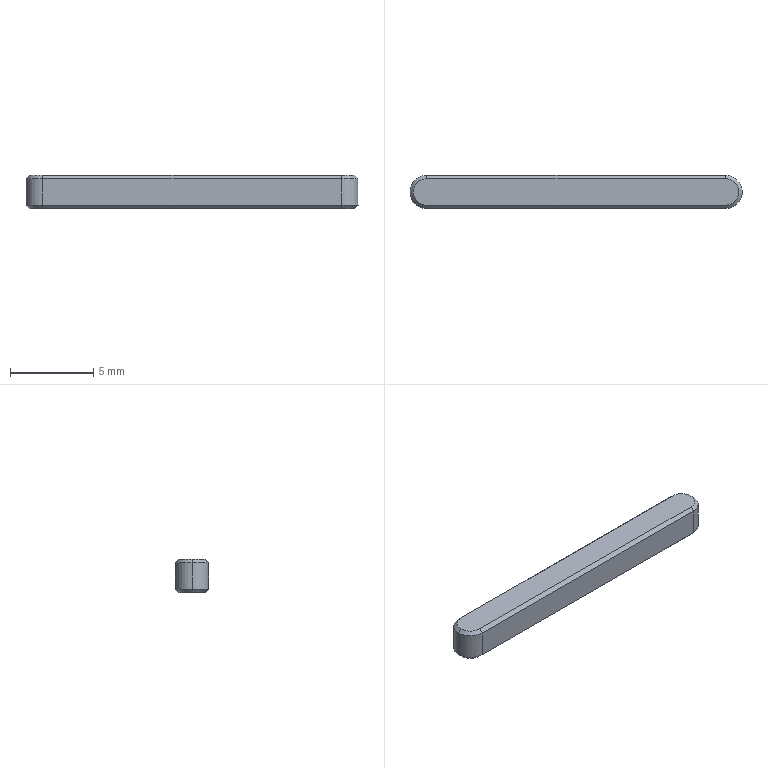Part | SolidWorks | features BaseBody 1 | 1 solid | 16 faces | box 20 x 2 x 2 mm | volume 76.609 mm3 | plane 8 | cone 5 | cylinder 3 | commonest cylinder face diameters 2 x3
STEP:
#1=CARTESIAN_POINT('',(-9.8,0.,2.));
#2=VERTEX_POINT('',#1);
#3=CARTESIAN_POINT('',(-9.,-0.8,2.));
#4=VERTEX_POINT('',#3);
#5=CARTESIAN_POINT('',(-9.,0.,2.));
#6=DIRECTION('',(0.,0.,1.));
#7=DIRECTION('',(-1.,0.,0.));
#8=AXIS2_PLACEMENT_3D('',#5,#6,#7);
#9=CIRCLE('',#8,0.8);
#10=EDGE_CURVE('',#2,#4,#9,.T.);
#11=ORIENTED_EDGE('',*,*,#10,.F.);
#12=CARTESIAN_POINT('',(-10.,0.,1.8));
#13=VERTEX_POINT('',#12);
#14=CARTESIAN_POINT('',(-10.,0.,1.8));
#15=DIRECTION('',(-0.7071,0.,-0.7071));
#16=VECTOR('',#15,1000.);
#17=LINE('',#14,#16);
#18=EDGE_CURVE('',#2,#13,#17,.T.);
#19=ORIENTED_EDGE('',*,*,#18,.T.);
#20=CARTESIAN_POINT('',(-9.,-1.,1.8));
#21=VERTEX_POINT('',#20);
#22=CARTESIAN_POINT('',(-9.,0.,1.8));
#23=DIRECTION('',(0.,0.,1.));
#24=DIRECTION('',(-1.,0.,0.));
#25=AXIS2_PLACEMENT_3D('',#22,#23,#24);
#26=CIRCLE('',#25,1.);
#27=EDGE_CURVE('',#13,#21,#26,.T.);
#28=ORIENTED_EDGE('',*,*,#27,.T.);
#29=CARTESIAN_POINT('',(-9.,-0.8,2.));
#30=DIRECTION('',(0.,-0.7071,-0.7071));
#31=VECTOR('',#30,1000.);
#32=LINE('',#29,#31);
#33=EDGE_CURVE('',#4,#21,#32,.T.);
#34=ORIENTED_EDGE('',*,*,#33,.F.);
#35=EDGE_LOOP('',(#11,#19,#28,#34));
#36=FACE_OUTER_BOUND('',#35,.T.);
#37=CARTESIAN_POINT('',(-9.,0.,1.8));
#38=DIRECTION('',(0.,0.,-1.));
#39=DIRECTION('',(-1.,0.,0.));
#40=AXIS2_PLACEMENT_3D('',#37,#38,#39);
#41=CONICAL_SURFACE('',#40,1.,0.7854);
#42=ADVANCED_FACE('',(#36),#41,.T.);
#43=ORIENTED_EDGE('',*,*,#27,.F.);
#44=CARTESIAN_POINT('',(-10.,0.,0.2));
#45=VERTEX_POINT('',#44);
#46=CARTESIAN_POINT('',(-10.,0.,2.));
#47=DIRECTION('',(0.,0.,-1.));
#48=VECTOR('',#47,1000.);
#49=LINE('',#46,#48);
#50=EDGE_CURVE('',#13,#45,#49,.T.);
#51=ORIENTED_EDGE('',*,*,#50,.T.);
#52=CARTESIAN_POINT('',(-9.,-1.,0.2));
#53=VERTEX_POINT('',#52);
#54=CARTESIAN_POINT('',(-9.,0.,0.2));
#55=DIRECTION('',(0.,0.,-1.));
#56=DIRECTION('',(1.,0.,0.));
#57=AXIS2_PLACEMENT_3D('',#54,#55,#56);
#58=CIRCLE('',#57,1.);
#59=EDGE_CURVE('',#53,#45,#58,.T.);
#60=ORIENTED_EDGE('',*,*,#59,.F.);
#61=CARTESIAN_POINT('',(-9.,-1.,2.));
#62=DIRECTION('',(0.,0.,1.));
#63=VECTOR('',#62,1000.);
#64=LINE('',#61,#63);
#65=EDGE_CURVE('',#53,#21,#64,.T.);
#66=ORIENTED_EDGE('',*,*,#65,.T.);
#67=EDGE_LOOP('',(#43,#51,#60,#66));
#68=FACE_OUTER_BOUND('',#67,.T.);
#69=CARTESIAN_POINT('',(-9.,0.,2.));
#70=DIRECTION('',(0.,0.,-1.));
#71=DIRECTION('',(-1.,0.,0.));
#72=AXIS2_PLACEMENT_3D('',#69,#70,#71);
#73=CYLINDRICAL_SURFACE('',#72,1.);
#74=ADVANCED_FACE('',(#68),#73,.T.);
#75=CARTESIAN_POINT('',(-9.,0.8,2.));
#76=VERTEX_POINT('',#75);
#77=CARTESIAN_POINT('',(-9.,0.,2.));
#78=DIRECTION('',(0.,0.,1.));
#79=DIRECTION('',(-1.,0.,0.));
#80=AXIS2_PLACEMENT_3D('',#77,#78,#79);
#81=CIRCLE('',#80,0.8);
#82=EDGE_CURVE('',#76,#2,#81,.T.);
#83=ORIENTED_EDGE('',*,*,#82,.T.);
#84=ORIENTED_EDGE('',*,*,#10,.T.);
#85=CARTESIAN_POINT('',(9.,-0.8,2.));
#86=VERTEX_POINT('',#85);
#87=CARTESIAN_POINT('',(-9.,-0.8,2.));
#88=DIRECTION('',(1.,0.,0.));
#89=VECTOR('',#88,1000.);
#90=LINE('',#87,#89);
#91=EDGE_CURVE('',#4,#86,#90,.T.);
#92=ORIENTED_EDGE('',*,*,#91,.T.);
#93=CARTESIAN_POINT('',(9.,0.8,2.));
#94=VERTEX_POINT('',#93);
#95=CARTESIAN_POINT('',(9.,0.,2.));
#96=DIRECTION('',(0.,0.,1.));
#97=DIRECTION('',(0.,1.,0.));
#98=AXIS2_PLACEMENT_3D('',#95,#96,#97);
#99=CIRCLE('',#98,0.8);
#100=EDGE_CURVE('',#86,#94,#99,.T.);
#101=ORIENTED_EDGE('',*,*,#100,.T.);
#102=CARTESIAN_POINT('',(-9.,0.8,2.));
#103=DIRECTION('',(-1.,0.,0.));
#104=VECTOR('',#103,1000.);
#105=LINE('',#102,#104);
#106=EDGE_CURVE('',#94,#76,#105,.T.);
#107=ORIENTED_EDGE('',*,*,#106,.T.);
#108=EDGE_LOOP('',(#83,#84,#92,#101,#107));
#109=FACE_OUTER_BOUND('',#108,.T.);
#110=CARTESIAN_POINT('',(-9.,0.,2.));
#111=DIRECTION('',(0.,0.,1.));
#112=DIRECTION('',(1.,0.,0.));
#113=AXIS2_PLACEMENT_3D('',#110,#111,#112);
#114=PLANE('',#113);
#115=ADVANCED_FACE('',(#109),#114,.T.);
#116=CARTESIAN_POINT('',(9.,-1.,1.8));
#117=VERTEX_POINT('',#116);
#118=CARTESIAN_POINT('',(9.,-0.8,2.));
#119=DIRECTION('',(0.,0.7071,0.7071));
#120=VECTOR('',#119,1000.);
#121=LINE('',#118,#120);
#122=EDGE_CURVE('',#117,#86,#121,.T.);
#123=ORIENTED_EDGE('',*,*,#122,.T.);
#124=ORIENTED_EDGE('',*,*,#91,.F.);
#125=ORIENTED_EDGE('',*,*,#33,.T.);
#126=CARTESIAN_POINT('',(-9.,-1.,1.8));
#127=DIRECTION('',(1.,0.,0.));
#128=VECTOR('',#127,1000.);
#129=LINE('',#126,#128);
#130=EDGE_CURVE('',#21,#117,#129,.T.);
#131=ORIENTED_EDGE('',*,*,#130,.T.);
#132=EDGE_LOOP('',(#123,#124,#125,#131));
#133=FACE_OUTER_BOUND('',#132,.T.);
#134=CARTESIAN_POINT('',(-9.,-0.8,2.));
#135=DIRECTION('',(0.,-0.7071,0.7071));
#136=DIRECTION('',(0.,-0.7071,-0.7071));
#137=AXIS2_PLACEMENT_3D('',#134,#135,#136);
#138=PLANE('',#137);
#139=ADVANCED_FACE('',(#133),#138,.T.);
#140=ORIENTED_EDGE('',*,*,#18,.F.);
#141=ORIENTED_EDGE('',*,*,#82,.F.);
#142=CARTESIAN_POINT('',(-9.,1.,1.8));
#143=VERTEX_POINT('',#142);
#144=CARTESIAN_POINT('',(-9.,498991.,-498988.2));
#145=DIRECTION('',(0.,0.7071,-0.7071));
#146=VECTOR('',#145,1000.);
#147=LINE('',#144,#146);
#148=EDGE_CURVE('',#76,#143,#147,.T.);
#149=ORIENTED_EDGE('',*,*,#148,.T.);
#150=CARTESIAN_POINT('',(-9.,0.,1.8));
#151=DIRECTION('',(0.,0.,1.));
#152=DIRECTION('',(-1.,0.,0.));
#153=AXIS2_PLACEMENT_3D('',#150,#151,#152);
#154=CIRCLE('',#153,1.);
#155=EDGE_CURVE('',#143,#13,#154,.T.);
#156=ORIENTED_EDGE('',*,*,#155,.T.);
#157=EDGE_LOOP('',(#140,#141,#149,#156));
#158=FACE_OUTER_BOUND('',#157,.T.);
#159=CARTESIAN_POINT('',(-9.,0.,1.8));
#160=DIRECTION('',(0.,0.,-1.));
#161=DIRECTION('',(-1.,0.,0.));
#162=AXIS2_PLACEMENT_3D('',#159,#160,#161);
#163=CONICAL_SURFACE('',#162,1.,0.7854);
#164=ADVANCED_FACE('',(#158),#163,.T.);
#165=ORIENTED_EDGE('',*,*,#148,.F.);
#166=ORIENTED_EDGE('',*,*,#106,.F.);
#167=CARTESIAN_POINT('',(9.,1.,1.8));
#168=VERTEX_POINT('',#167);
#169=CARTESIAN_POINT('',(9.,0.8,2.));
#170=DIRECTION('',(0.,0.7071,-0.7071));
#171=VECTOR('',#170,1000.);
#172=LINE('',#169,#171);
#173=EDGE_CURVE('',#94,#168,#172,.T.);
#174=ORIENTED_EDGE('',*,*,#173,.T.);
#175=CARTESIAN_POINT('',(-9.,1.,1.8));
#176=DIRECTION('',(-1.,0.,0.));
#177=VECTOR('',#176,1000.);
#178=LINE('',#175,#177);
#179=EDGE_CURVE('',#168,#143,#178,.T.);
#180=ORIENTED_EDGE('',*,*,#179,.T.);
#181=EDGE_LOOP('',(#165,#166,#174,#180));
#182=FACE_OUTER_BOUND('',#181,.T.);
#183=CARTESIAN_POINT('',(-9.,0.8,2.));
#184=DIRECTION('',(0.,0.7071,0.7071));
#185=DIRECTION('',(0.,-0.7071,0.7071));
#186=AXIS2_PLACEMENT_3D('',#183,#184,#185);
#187=PLANE('',#186);
#188=ADVANCED_FACE('',(#182),#187,.T.);
#189=ORIENTED_EDGE('',*,*,#173,.F.);
#190=ORIENTED_EDGE('',*,*,#100,.F.);
#191=ORIENTED_EDGE('',*,*,#122,.F.);
#192=CARTESIAN_POINT('',(9.,0.,1.8));
#193=DIRECTION('',(0.,0.,1.));
#194=DIRECTION('',(-1.,0.,0.));
#195=AXIS2_PLACEMENT_3D('',#192,#193,#194);
#196=CIRCLE('',#195,1.);
#197=EDGE_CURVE('',#117,#168,#196,.T.);
#198=ORIENTED_EDGE('',*,*,#197,.T.);
#199=EDGE_LOOP('',(#189,#190,#191,#198));
#200=FACE_OUTER_BOUND('',#199,.T.);
#201=CARTESIAN_POINT('',(9.,0.,1.8));
#202=DIRECTION('',(0.,0.,-1.));
#203=DIRECTION('',(0.,1.,0.));
#204=AXIS2_PLACEMENT_3D('',#201,#202,#203);
#205=CONICAL_SURFACE('',#204,1.,0.7854);
#206=ADVANCED_FACE('',(#200),#205,.T.);
#207=ORIENTED_EDGE('',*,*,#130,.F.);
#208=ORIENTED_EDGE('',*,*,#65,.F.);
#209=CARTESIAN_POINT('',(9.,-1.,0.2));
#210=VERTEX_POINT('',#209);
#211=CARTESIAN_POINT('',(-9.,-1.,0.2));
#212=DIRECTION('',(-1.,0.,0.));
#213=VECTOR('',#212,1000.);
#214=LINE('',#211,#213);
#215=EDGE_CURVE('',#210,#53,#214,.T.);
#216=ORIENTED_EDGE('',*,*,#215,.F.);
#217=CARTESIAN_POINT('',(9.,-1.,2.));
#218=DIRECTION('',(0.,0.,-1.));
#219=VECTOR('',#218,1000.);
#220=LINE('',#217,#219);
#221=EDGE_CURVE('',#117,#210,#220,.T.);
#222=ORIENTED_EDGE('',*,*,#221,.F.);
#223=EDGE_LOOP('',(#207,#208,#216,#222));
#224=FACE_OUTER_BOUND('',#223,.T.);
#225=CARTESIAN_POINT('',(-9.,-1.,2.));
#226=DIRECTION('',(0.,1.,0.));
#227=DIRECTION('',(0.,0.,1.));
#228=AXIS2_PLACEMENT_3D('',#225,#226,#227);
#229=PLANE('',#228);
#230=ADVANCED_FACE('',(#224),#229,.F.);
#231=ORIENTED_EDGE('',*,*,#50,.F.);
#232=ORIENTED_EDGE('',*,*,#155,.F.);
#233=CARTESIAN_POINT('',(-9.,1.,0.2));
#234=VERTEX_POINT('',#233);
#235=CARTESIAN_POINT('',(-9.,1.,2.));
#236=DIRECTION('',(0.,0.,-1.));
#237=VECTOR('',#236,1000.);
#238=LINE('',#235,#237);
#239=EDGE_CURVE('',#143,#234,#238,.T.);
#240=ORIENTED_EDGE('',*,*,#239,.T.);
#241=CARTESIAN_POINT('',(-9.,0.,0.2));
#242=DIRECTION('',(0.,0.,-1.));
#243=DIRECTION('',(1.,0.,0.));
#244=AXIS2_PLACEMENT_3D('',#241,#242,#243);
#245=CIRCLE('',#244,1.);
#246=EDGE_CURVE('',#45,#234,#245,.T.);
#247=ORIENTED_EDGE('',*,*,#246,.F.);
#248=EDGE_LOOP('',(#231,#232,#240,#247));
#249=FACE_OUTER_BOUND('',#248,.T.);
#250=CARTESIAN_POINT('',(-9.,0.,2.));
#251=DIRECTION('',(0.,0.,-1.));
#252=DIRECTION('',(-1.,0.,0.));
#253=AXIS2_PLACEMENT_3D('',#250,#251,#252);
#254=CYLINDRICAL_SURFACE('',#253,1.);
#255=ADVANCED_FACE('',(#249),#254,.T.);
#256=ORIENTED_EDGE('',*,*,#179,.F.);
#257=CARTESIAN_POINT('',(9.,1.,0.2));
#258=VERTEX_POINT('',#257);
#259=CARTESIAN_POINT('',(9.,1.,2.));
#260=DIRECTION('',(0.,0.,1.));
#261=VECTOR('',#260,1000.);
#262=LINE('',#259,#261);
#263=EDGE_CURVE('',#258,#168,#262,.T.);
#264=ORIENTED_EDGE('',*,*,#263,.F.);
#265=CARTESIAN_POINT('',(-9.,1.,0.2));
#266=DIRECTION('',(1.,0.,0.));
#267=VECTOR('',#266,1000.);
#268=LINE('',#265,#267);
#269=EDGE_CURVE('',#234,#258,#268,.T.);
#270=ORIENTED_EDGE('',*,*,#269,.F.);
#271=ORIENTED_EDGE('',*,*,#239,.F.);
#272=EDGE_LOOP('',(#256,#264,#270,#271));
#273=FACE_OUTER_BOUND('',#272,.T.);
#274=CARTESIAN_POINT('',(-9.,1.,2.));
#275=DIRECTION('',(0.,-1.,0.));
#276=DIRECTION('',(0.,0.,-1.));
#277=AXIS2_PLACEMENT_3D('',#274,#275,#276);
#278=PLANE('',#277);
#279=ADVANCED_FACE('',(#273),#278,.F.);
#280=ORIENTED_EDGE('',*,*,#221,.T.);
#281=CARTESIAN_POINT('',(9.,0.,0.2));
#282=DIRECTION('',(0.,0.,1.));
#283=DIRECTION('',(-1.,0.,0.));
#284=AXIS2_PLACEMENT_3D('',#281,#282,#283);
#285=CIRCLE('',#284,1.);
#286=EDGE_CURVE('',#210,#258,#285,.T.);
#287=ORIENTED_EDGE('',*,*,#286,.T.);
#288=ORIENTED_EDGE('',*,*,#263,.T.);
#289=ORIENTED_EDGE('',*,*,#197,.F.);
#290=EDGE_LOOP('',(#280,#287,#288,#289));
#291=FACE_OUTER_BOUND('',#290,.T.);
#292=CARTESIAN_POINT('',(9.,0.,2.));
#293=DIRECTION('',(0.,0.,-1.));
#294=DIRECTION('',(-1.,0.,0.));
#295=AXIS2_PLACEMENT_3D('',#292,#293,#294);
#296=CYLINDRICAL_SURFACE('',#295,1.);
#297=ADVANCED_FACE('',(#291),#296,.T.);
#298=CARTESIAN_POINT('',(9.,-0.8,0.));
#299=VERTEX_POINT('',#298);
#300=CARTESIAN_POINT('',(-9.,-0.8,0.));
#301=VERTEX_POINT('',#300);
#302=CARTESIAN_POINT('',(-9.,-0.8,0.));
#303=DIRECTION('',(-1.,0.,0.));
#304=VECTOR('',#303,1000.);
#305=LINE('',#302,#304);
#306=EDGE_CURVE('',#299,#301,#305,.T.);
#307=ORIENTED_EDGE('',*,*,#306,.F.);
#308=CARTESIAN_POINT('',(9.,-1.,0.2));
#309=DIRECTION('',(0.,0.7071,-0.7071));
#310=VECTOR('',#309,1000.);
#311=LINE('',#308,#310);
#312=EDGE_CURVE('',#210,#299,#311,.T.);
#313=ORIENTED_EDGE('',*,*,#312,.F.);
#314=ORIENTED_EDGE('',*,*,#215,.T.);
#315=CARTESIAN_POINT('',(-9.,-499000.8,499000.));
#316=DIRECTION('',(0.,-0.7071,0.7071));
#317=VECTOR('',#316,1000.);
#318=LINE('',#315,#317);
#319=EDGE_CURVE('',#301,#53,#318,.T.);
#320=ORIENTED_EDGE('',*,*,#319,.F.);
#321=EDGE_LOOP('',(#307,#313,#314,#320));
#322=FACE_OUTER_BOUND('',#321,.T.);
#323=CARTESIAN_POINT('',(-9.,-1.,0.2));
#324=DIRECTION('',(0.,0.7071,0.7071));
#325=DIRECTION('',(0.,-0.7071,0.7071));
#326=AXIS2_PLACEMENT_3D('',#323,#324,#325);
#327=PLANE('',#326);
#328=ADVANCED_FACE('',(#322),#327,.F.);
#329=CARTESIAN_POINT('',(-9.,0.8,0.));
#330=VERTEX_POINT('',#329);
#331=CARTESIAN_POINT('',(9.,0.8,0.));
#332=VERTEX_POINT('',#331);
#333=CARTESIAN_POINT('',(-9.,0.8,0.));
#334=DIRECTION('',(1.,0.,0.));
#335=VECTOR('',#334,1000.);
#336=LINE('',#333,#335);
#337=EDGE_CURVE('',#330,#332,#336,.T.);
#338=ORIENTED_EDGE('',*,*,#337,.F.);
#339=CARTESIAN_POINT('',(-9.,499000.8,499000.));
#340=DIRECTION('',(0.,-0.7071,-0.7071));
#341=VECTOR('',#340,1000.);
#342=LINE('',#339,#341);
#343=EDGE_CURVE('',#234,#330,#342,.T.);
#344=ORIENTED_EDGE('',*,*,#343,.F.);
#345=ORIENTED_EDGE('',*,*,#269,.T.);
#346=CARTESIAN_POINT('',(9.,1.,0.2));
#347=DIRECTION('',(0.,0.7071,0.7071));
#348=VECTOR('',#347,1000.);
#349=LINE('',#346,#348);
#350=EDGE_CURVE('',#332,#258,#349,.T.);
#351=ORIENTED_EDGE('',*,*,#350,.F.);
#352=EDGE_LOOP('',(#338,#344,#345,#351));
#353=FACE_OUTER_BOUND('',#352,.T.);
#354=CARTESIAN_POINT('',(-9.,1.,0.2));
#355=DIRECTION('',(0.,-0.7071,0.7071));
#356=DIRECTION('',(0.,-0.7071,-0.7071));
#357=AXIS2_PLACEMENT_3D('',#354,#355,#356);
#358=PLANE('',#357);
#359=ADVANCED_FACE('',(#353),#358,.F.);
#360=ORIENTED_EDGE('',*,*,#350,.T.);
#361=ORIENTED_EDGE('',*,*,#286,.F.);
#362=ORIENTED_EDGE('',*,*,#312,.T.);
#363=CARTESIAN_POINT('',(9.,0.,0.));
#364=DIRECTION('',(0.,0.,1.));
#365=DIRECTION('',(0.,-1.,0.));
#366=AXIS2_PLACEMENT_3D('',#363,#364,#365);
#367=CIRCLE('',#366,0.8);
#368=EDGE_CURVE('',#299,#332,#367,.T.);
#369=ORIENTED_EDGE('',*,*,#368,.T.);
#370=EDGE_LOOP('',(#360,#361,#362,#369));
#371=FACE_OUTER_BOUND('',#370,.T.);
#372=CARTESIAN_POINT('',(9.,0.,0.2));
#373=DIRECTION('',(0.,0.,1.));
#374=DIRECTION('',(0.,-1.,0.));
#375=AXIS2_PLACEMENT_3D('',#372,#373,#374);
#376=CONICAL_SURFACE('',#375,1.,0.7854);
#377=ADVANCED_FACE('',(#371),#376,.T.);
#378=ORIENTED_EDGE('',*,*,#337,.T.);
#379=ORIENTED_EDGE('',*,*,#368,.F.);
#380=ORIENTED_EDGE('',*,*,#306,.T.);
#381=CARTESIAN_POINT('',(-9.,0.,0.));
#382=DIRECTION('',(0.,0.,1.));
#383=DIRECTION('',(1.,0.,0.));
#384=AXIS2_PLACEMENT_3D('',#381,#382,#383);
#385=CIRCLE('',#384,0.8);
#386=EDGE_CURVE('',#330,#301,#385,.T.);
#387=ORIENTED_EDGE('',*,*,#386,.F.);
#388=EDGE_LOOP('',(#378,#379,#380,#387));
#389=FACE_OUTER_BOUND('',#388,.T.);
#390=CARTESIAN_POINT('',(-9.,0.,0.));
#391=DIRECTION('',(0.,0.,1.));
#392=DIRECTION('',(1.,0.,0.));
#393=AXIS2_PLACEMENT_3D('',#390,#391,#392);
#394=PLANE('',#393);
#395=ADVANCED_FACE('',(#389),#394,.F.);
#396=ORIENTED_EDGE('',*,*,#343,.T.);
#397=ORIENTED_EDGE('',*,*,#386,.T.);
#398=ORIENTED_EDGE('',*,*,#319,.T.);
#399=ORIENTED_EDGE('',*,*,#59,.T.);
#400=ORIENTED_EDGE('',*,*,#246,.T.);
#401=EDGE_LOOP('',(#396,#397,#398,#399,#400));
#402=FACE_OUTER_BOUND('',#401,.T.);
#403=CARTESIAN_POINT('',(-9.,0.,0.2));
#404=DIRECTION('',(0.,0.,1.));
#405=DIRECTION('',(1.,0.,0.));
#406=AXIS2_PLACEMENT_3D('',#403,#404,#405);
#407=CONICAL_SURFACE('',#406,1.,0.7854);
#408=ADVANCED_FACE('',(#402),#407,.T.);
#409=CLOSED_SHELL('',(#42,#74,#115,#139,#164,#188,#206,#230,#255,#279,#297,#328,#359,#377,#395,#408));
#410=MANIFOLD_SOLID_BREP('',#409);
#411=CARTESIAN_POINT('',(0.,0.,0.));
#412=DIRECTION('',(0.,0.,1.));
#413=DIRECTION('',(1.,0.,0.));
#414=AXIS2_PLACEMENT_3D('',#411,#412,#413);
#415=(LENGTH_UNIT()NAMED_UNIT(*)SI_UNIT(.MILLI.,.METRE.));
#416=UNCERTAINTY_MEASURE_WITH_UNIT(LENGTH_MEASURE(0.00001),#415,'','');
#417=(NAMED_UNIT(*)PLANE_ANGLE_UNIT()SI_UNIT($,.RADIAN.));
#418=(NAMED_UNIT(*)SI_UNIT($,.STERADIAN.)SOLID_ANGLE_UNIT());
#419=(GEOMETRIC_REPRESENTATION_CONTEXT(3)GLOBAL_UNCERTAINTY_ASSIGNED_CONTEXT((#416))GLOBAL_UNIT_ASSIGNED_CONTEXT((#415,#417,#418))REPRESENTATION_CONTEXT('',''));
#420=ADVANCED_BREP_SHAPE_REPRESENTATION('',(#410,#414),#419);